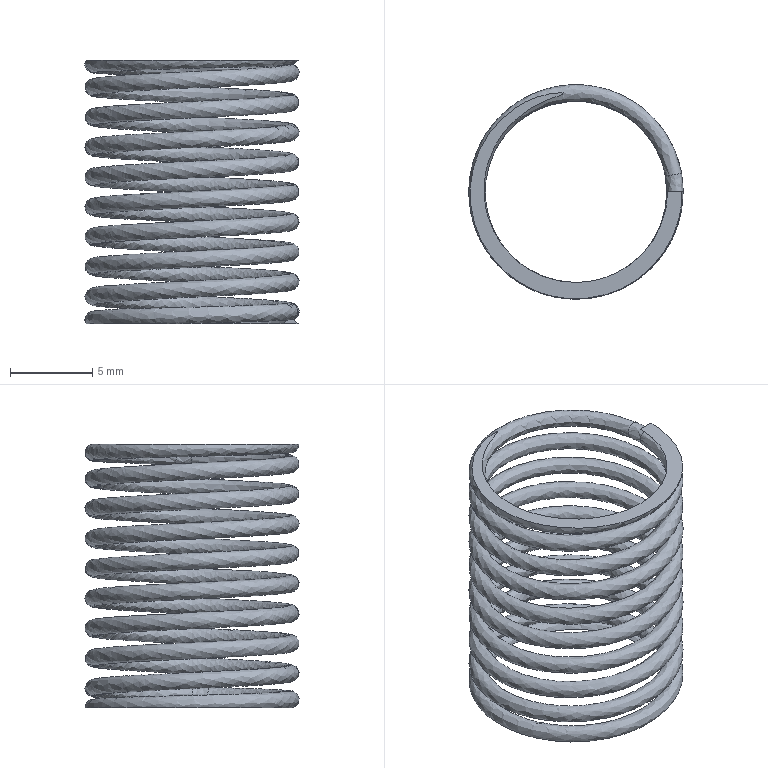Part | NX | features SPLINE_LAW 3, BRIDGE_CURVE 2, DATUM_CSYS 2, DATUM_PLANE 2, TRIM BODY 2, ABSOLUTE_DATUM_AXIS 1, ABSOLUTE_DATUM_PLANE 1, DATUM_ON_PATH 1, FLEXIBLE_PART 1, FSET 1, SKETCH 1, SKIN 1 | 1 solid | 9 faces | volume 283.448 mm3 | spline 5 | plane 4